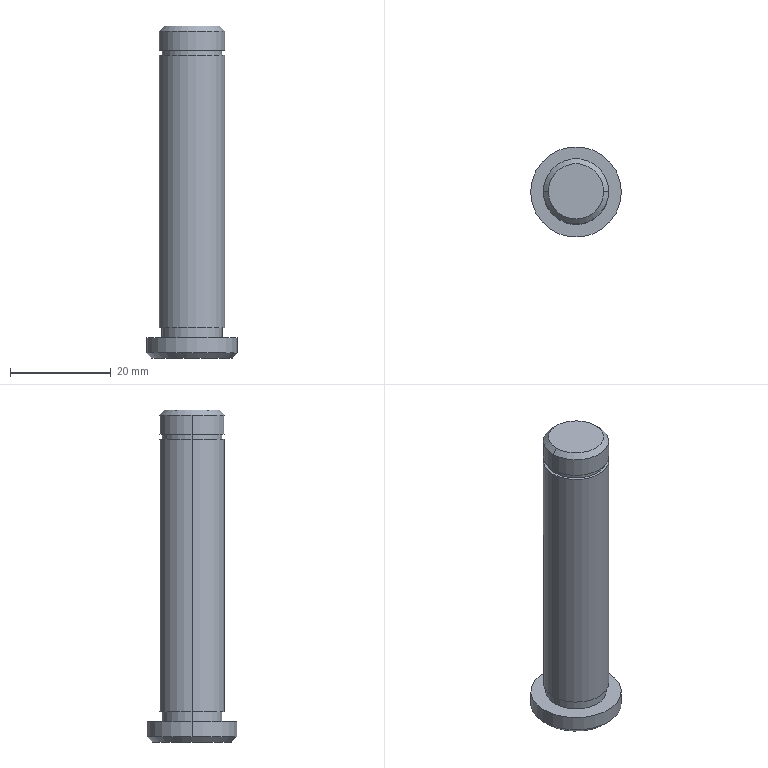Part | SolidWorks | features ICE 4, Chamfer 1, Extrusion 1 | 1 solid | 20 faces | box 18 x 18 x 66 mm | volume 9140 mm3 | cylinder 10 | plane 6 | cone 4 | commonest cylinder face diameters 13 x4 11.9 x2 12 x2 18 x2
STEP:
#1=CARTESIAN_POINT('',(5.5,0.,66.));
#2=VERTEX_POINT('',#1);
#3=CARTESIAN_POINT('',(-5.5,0.,66.));
#4=VERTEX_POINT('',#3);
#5=CARTESIAN_POINT('',(0.,0.,66.));
#6=DIRECTION('',(0.,0.,1.));
#7=DIRECTION('',(1.,0.,0.));
#8=AXIS2_PLACEMENT_3D('',#5,#6,#7);
#9=CIRCLE('',#8,5.5);
#10=EDGE_CURVE('',#2,#4,#9,.T.);
#11=ORIENTED_EDGE('',*,*,#10,.F.);
#12=CARTESIAN_POINT('',(6.5,0.,65.));
#13=VERTEX_POINT('',#12);
#14=CARTESIAN_POINT('',(5.5,0.,66.));
#15=DIRECTION('',(0.7071,0.,-0.7071));
#16=VECTOR('',#15,1000.);
#17=LINE('',#14,#16);
#18=EDGE_CURVE('',#2,#13,#17,.T.);
#19=ORIENTED_EDGE('',*,*,#18,.T.);
#20=CARTESIAN_POINT('',(-6.5,0.,65.));
#21=VERTEX_POINT('',#20);
#22=CARTESIAN_POINT('',(0.,0.,65.));
#23=DIRECTION('',(0.,0.,-1.));
#24=DIRECTION('',(1.,0.,0.));
#25=AXIS2_PLACEMENT_3D('',#22,#23,#24);
#26=CIRCLE('',#25,6.5);
#27=EDGE_CURVE('',#21,#13,#26,.T.);
#28=ORIENTED_EDGE('',*,*,#27,.F.);
#29=CARTESIAN_POINT('',(-5.5,0.,66.));
#30=DIRECTION('',(-0.7071,0.,-0.7071));
#31=VECTOR('',#30,1000.);
#32=LINE('',#29,#31);
#33=EDGE_CURVE('',#4,#21,#32,.T.);
#34=ORIENTED_EDGE('',*,*,#33,.F.);
#35=EDGE_LOOP('',(#11,#19,#28,#34));
#36=FACE_OUTER_BOUND('',#35,.T.);
#37=CARTESIAN_POINT('',(0.,0.,66.));
#38=DIRECTION('',(0.,0.,-1.));
#39=DIRECTION('',(-1.,0.,0.));
#40=AXIS2_PLACEMENT_3D('',#37,#38,#39);
#41=CONICAL_SURFACE('',#40,5.5,0.7854);
#42=ADVANCED_FACE('',(#36),#41,.T.);
#43=CARTESIAN_POINT('',(-8.,0.,0.));
#44=VERTEX_POINT('',#43);
#45=CARTESIAN_POINT('',(8.,0.,0.));
#46=VERTEX_POINT('',#45);
#47=CARTESIAN_POINT('',(0.,0.,0.));
#48=DIRECTION('',(0.,0.,-1.));
#49=DIRECTION('',(1.,0.,0.));
#50=AXIS2_PLACEMENT_3D('',#47,#48,#49);
#51=CIRCLE('',#50,8.);
#52=EDGE_CURVE('',#44,#46,#51,.T.);
#53=ORIENTED_EDGE('',*,*,#52,.F.);
#54=CARTESIAN_POINT('',(-9.,0.,1.));
#55=VERTEX_POINT('',#54);
#56=CARTESIAN_POINT('',(-9.,0.,1.));
#57=DIRECTION('',(-0.7071,0.,0.7071));
#58=VECTOR('',#57,1000.);
#59=LINE('',#56,#58);
#60=EDGE_CURVE('',#44,#55,#59,.T.);
#61=ORIENTED_EDGE('',*,*,#60,.T.);
#62=CARTESIAN_POINT('',(9.,0.,1.));
#63=VERTEX_POINT('',#62);
#64=CARTESIAN_POINT('',(0.,0.,1.));
#65=DIRECTION('',(0.,0.,1.));
#66=DIRECTION('',(1.,0.,0.));
#67=AXIS2_PLACEMENT_3D('',#64,#65,#66);
#68=CIRCLE('',#67,9.);
#69=EDGE_CURVE('',#63,#55,#68,.T.);
#70=ORIENTED_EDGE('',*,*,#69,.F.);
#71=CARTESIAN_POINT('',(9.,0.,1.));
#72=DIRECTION('',(0.7071,0.,0.7071));
#73=VECTOR('',#72,1000.);
#74=LINE('',#71,#73);
#75=EDGE_CURVE('',#46,#63,#74,.T.);
#76=ORIENTED_EDGE('',*,*,#75,.F.);
#77=EDGE_LOOP('',(#53,#61,#70,#76));
#78=FACE_OUTER_BOUND('',#77,.T.);
#79=CARTESIAN_POINT('',(0.,0.,1.));
#80=DIRECTION('',(0.,0.,1.));
#81=DIRECTION('',(1.,0.,0.));
#82=AXIS2_PLACEMENT_3D('',#79,#80,#81);
#83=CONICAL_SURFACE('',#82,9.,0.7854);
#84=ADVANCED_FACE('',(#78),#83,.T.);
#85=ORIENTED_EDGE('',*,*,#27,.T.);
#86=CARTESIAN_POINT('',(6.5,0.,61.2));
#87=VERTEX_POINT('',#86);
#88=CARTESIAN_POINT('',(6.5,0.,150.385));
#89=DIRECTION('',(0.,0.,-1.));
#90=VECTOR('',#89,1000.);
#91=LINE('',#88,#90);
#92=EDGE_CURVE('',#13,#87,#91,.T.);
#93=ORIENTED_EDGE('',*,*,#92,.T.);
#94=CARTESIAN_POINT('',(-6.5,0.,61.2));
#95=VERTEX_POINT('',#94);
#96=CARTESIAN_POINT('',(0.,0.,61.2));
#97=DIRECTION('',(0.,0.,1.));
#98=DIRECTION('',(1.,0.,0.));
#99=AXIS2_PLACEMENT_3D('',#96,#97,#98);
#100=CIRCLE('',#99,6.5);
#101=EDGE_CURVE('',#87,#95,#100,.T.);
#102=ORIENTED_EDGE('',*,*,#101,.T.);
#103=CARTESIAN_POINT('',(-6.5,0.,150.385));
#104=DIRECTION('',(0.,0.,-1.));
#105=VECTOR('',#104,1000.);
#106=LINE('',#103,#105);
#107=EDGE_CURVE('',#21,#95,#106,.T.);
#108=ORIENTED_EDGE('',*,*,#107,.F.);
#109=EDGE_LOOP('',(#85,#93,#102,#108));
#110=FACE_OUTER_BOUND('',#109,.T.);
#111=CARTESIAN_POINT('',(0.,0.,150.385));
#112=DIRECTION('',(0.,0.,-1.));
#113=DIRECTION('',(-1.,0.,0.));
#114=AXIS2_PLACEMENT_3D('',#111,#112,#113);
#115=CYLINDRICAL_SURFACE('',#114,6.5);
#116=ADVANCED_FACE('',(#110),#115,.T.);
#117=CARTESIAN_POINT('',(5.95,0.,61.2));
#118=VERTEX_POINT('',#117);
#119=CARTESIAN_POINT('',(-5.95,0.,61.2));
#120=VERTEX_POINT('',#119);
#121=CARTESIAN_POINT('',(0.,0.,61.2));
#122=DIRECTION('',(0.,0.,1.));
#123=DIRECTION('',(1.,0.,0.));
#124=AXIS2_PLACEMENT_3D('',#121,#122,#123);
#125=CIRCLE('',#124,5.95);
#126=EDGE_CURVE('',#118,#120,#125,.T.);
#127=ORIENTED_EDGE('',*,*,#126,.F.);
#128=CARTESIAN_POINT('',(5.95,0.,60.2));
#129=VERTEX_POINT('',#128);
#130=CARTESIAN_POINT('',(5.95,0.,61.2));
#131=DIRECTION('',(0.,0.,-1.));
#132=VECTOR('',#131,1000.);
#133=LINE('',#130,#132);
#134=EDGE_CURVE('',#118,#129,#133,.T.);
#135=ORIENTED_EDGE('',*,*,#134,.T.);
#136=CARTESIAN_POINT('',(-5.95,0.,60.2));
#137=VERTEX_POINT('',#136);
#138=CARTESIAN_POINT('',(0.,0.,60.2));
#139=DIRECTION('',(0.,0.,1.));
#140=DIRECTION('',(1.,0.,0.));
#141=AXIS2_PLACEMENT_3D('',#138,#139,#140);
#142=CIRCLE('',#141,5.95);
#143=EDGE_CURVE('',#129,#137,#142,.T.);
#144=ORIENTED_EDGE('',*,*,#143,.T.);
#145=CARTESIAN_POINT('',(-5.95,0.,61.2));
#146=DIRECTION('',(0.,0.,-1.));
#147=VECTOR('',#146,1000.);
#148=LINE('',#145,#147);
#149=EDGE_CURVE('',#120,#137,#148,.T.);
#150=ORIENTED_EDGE('',*,*,#149,.F.);
#151=EDGE_LOOP('',(#127,#135,#144,#150));
#152=FACE_OUTER_BOUND('',#151,.T.);
#153=CARTESIAN_POINT('',(0.,0.,61.2));
#154=DIRECTION('',(0.,0.,-1.));
#155=DIRECTION('',(-1.,0.,0.));
#156=AXIS2_PLACEMENT_3D('',#153,#154,#155);
#157=CYLINDRICAL_SURFACE('',#156,5.95);
#158=ADVANCED_FACE('',(#152),#157,.T.);
#159=CARTESIAN_POINT('',(6.5,0.,60.2));
#160=VERTEX_POINT('',#159);
#161=CARTESIAN_POINT('',(-6.5,0.,60.2));
#162=VERTEX_POINT('',#161);
#163=CARTESIAN_POINT('',(0.,0.,60.2));
#164=DIRECTION('',(0.,0.,1.));
#165=DIRECTION('',(1.,0.,0.));
#166=AXIS2_PLACEMENT_3D('',#163,#164,#165);
#167=CIRCLE('',#166,6.5);
#168=EDGE_CURVE('',#160,#162,#167,.T.);
#169=ORIENTED_EDGE('',*,*,#168,.F.);
#170=CARTESIAN_POINT('',(6.5,0.,6.));
#171=VERTEX_POINT('',#170);
#172=CARTESIAN_POINT('',(6.5,0.,60.2));
#173=DIRECTION('',(0.,0.,-1.));
#174=VECTOR('',#173,1000.);
#175=LINE('',#172,#174);
#176=EDGE_CURVE('',#160,#171,#175,.T.);
#177=ORIENTED_EDGE('',*,*,#176,.T.);
#178=CARTESIAN_POINT('',(-6.5,0.,6.));
#179=VERTEX_POINT('',#178);
#180=CARTESIAN_POINT('',(0.,0.,6.));
#181=DIRECTION('',(0.,0.,1.));
#182=DIRECTION('',(1.,0.,0.));
#183=AXIS2_PLACEMENT_3D('',#180,#181,#182);
#184=CIRCLE('',#183,6.5);
#185=EDGE_CURVE('',#171,#179,#184,.T.);
#186=ORIENTED_EDGE('',*,*,#185,.T.);
#187=CARTESIAN_POINT('',(-6.5,0.,60.2));
#188=DIRECTION('',(0.,0.,-1.));
#189=VECTOR('',#188,1000.);
#190=LINE('',#187,#189);
#191=EDGE_CURVE('',#162,#179,#190,.T.);
#192=ORIENTED_EDGE('',*,*,#191,.F.);
#193=EDGE_LOOP('',(#169,#177,#186,#192));
#194=FACE_OUTER_BOUND('',#193,.T.);
#195=CARTESIAN_POINT('',(0.,0.,60.2));
#196=DIRECTION('',(0.,0.,-1.));
#197=DIRECTION('',(-1.,0.,0.));
#198=AXIS2_PLACEMENT_3D('',#195,#196,#197);
#199=CYLINDRICAL_SURFACE('',#198,6.5);
#200=ADVANCED_FACE('',(#194),#199,.T.);
#201=CARTESIAN_POINT('',(6.,0.,6.));
#202=VERTEX_POINT('',#201);
#203=CARTESIAN_POINT('',(-6.,0.,6.));
#204=VERTEX_POINT('',#203);
#205=CARTESIAN_POINT('',(0.,0.,6.));
#206=DIRECTION('',(0.,0.,1.));
#207=DIRECTION('',(1.,0.,0.));
#208=AXIS2_PLACEMENT_3D('',#205,#206,#207);
#209=CIRCLE('',#208,6.);
#210=EDGE_CURVE('',#202,#204,#209,.T.);
#211=ORIENTED_EDGE('',*,*,#210,.F.);
#212=CARTESIAN_POINT('',(6.,0.,4.));
#213=VERTEX_POINT('',#212);
#214=CARTESIAN_POINT('',(6.,0.,6.));
#215=DIRECTION('',(0.,0.,-1.));
#216=VECTOR('',#215,1000.);
#217=LINE('',#214,#216);
#218=EDGE_CURVE('',#202,#213,#217,.T.);
#219=ORIENTED_EDGE('',*,*,#218,.T.);
#220=CARTESIAN_POINT('',(-6.,0.,4.));
#221=VERTEX_POINT('',#220);
#222=CARTESIAN_POINT('',(0.,0.,4.));
#223=DIRECTION('',(0.,0.,1.));
#224=DIRECTION('',(1.,0.,0.));
#225=AXIS2_PLACEMENT_3D('',#222,#223,#224);
#226=CIRCLE('',#225,6.);
#227=EDGE_CURVE('',#213,#221,#226,.T.);
#228=ORIENTED_EDGE('',*,*,#227,.T.);
#229=CARTESIAN_POINT('',(-6.,0.,6.));
#230=DIRECTION('',(0.,0.,-1.));
#231=VECTOR('',#230,1000.);
#232=LINE('',#229,#231);
#233=EDGE_CURVE('',#204,#221,#232,.T.);
#234=ORIENTED_EDGE('',*,*,#233,.F.);
#235=EDGE_LOOP('',(#211,#219,#228,#234));
#236=FACE_OUTER_BOUND('',#235,.T.);
#237=CARTESIAN_POINT('',(0.,0.,6.));
#238=DIRECTION('',(0.,0.,-1.));
#239=DIRECTION('',(-1.,0.,0.));
#240=AXIS2_PLACEMENT_3D('',#237,#238,#239);
#241=CYLINDRICAL_SURFACE('',#240,6.);
#242=ADVANCED_FACE('',(#236),#241,.T.);
#243=CARTESIAN_POINT('',(9.,0.,4.));
#244=VERTEX_POINT('',#243);
#245=CARTESIAN_POINT('',(-9.,0.,4.));
#246=VERTEX_POINT('',#245);
#247=CARTESIAN_POINT('',(0.,0.,4.));
#248=DIRECTION('',(0.,0.,1.));
#249=DIRECTION('',(1.,0.,0.));
#250=AXIS2_PLACEMENT_3D('',#247,#248,#249);
#251=CIRCLE('',#250,9.);
#252=EDGE_CURVE('',#244,#246,#251,.T.);
#253=ORIENTED_EDGE('',*,*,#252,.F.);
#254=CARTESIAN_POINT('',(9.,0.,4.));
#255=DIRECTION('',(0.,0.,-1.));
#256=VECTOR('',#255,1000.);
#257=LINE('',#254,#256);
#258=EDGE_CURVE('',#244,#63,#257,.T.);
#259=ORIENTED_EDGE('',*,*,#258,.T.);
#260=ORIENTED_EDGE('',*,*,#69,.T.);
#261=CARTESIAN_POINT('',(-9.,0.,4.));
#262=DIRECTION('',(0.,0.,-1.));
#263=VECTOR('',#262,1000.);
#264=LINE('',#261,#263);
#265=EDGE_CURVE('',#246,#55,#264,.T.);
#266=ORIENTED_EDGE('',*,*,#265,.F.);
#267=EDGE_LOOP('',(#253,#259,#260,#266));
#268=FACE_OUTER_BOUND('',#267,.T.);
#269=CARTESIAN_POINT('',(0.,0.,4.));
#270=DIRECTION('',(0.,0.,-1.));
#271=DIRECTION('',(-1.,0.,0.));
#272=AXIS2_PLACEMENT_3D('',#269,#270,#271);
#273=CYLINDRICAL_SURFACE('',#272,9.);
#274=ADVANCED_FACE('',(#268),#273,.T.);
#275=ORIENTED_EDGE('',*,*,#258,.F.);
#276=CARTESIAN_POINT('',(0.,0.,4.));
#277=DIRECTION('',(0.,0.,1.));
#278=DIRECTION('',(1.,0.,0.));
#279=AXIS2_PLACEMENT_3D('',#276,#277,#278);
#280=CIRCLE('',#279,9.);
#281=EDGE_CURVE('',#246,#244,#280,.T.);
#282=ORIENTED_EDGE('',*,*,#281,.F.);
#283=ORIENTED_EDGE('',*,*,#265,.T.);
#284=CARTESIAN_POINT('',(0.,0.,1.));
#285=DIRECTION('',(0.,0.,1.));
#286=DIRECTION('',(1.,0.,0.));
#287=AXIS2_PLACEMENT_3D('',#284,#285,#286);
#288=CIRCLE('',#287,9.);
#289=EDGE_CURVE('',#55,#63,#288,.T.);
#290=ORIENTED_EDGE('',*,*,#289,.T.);
#291=EDGE_LOOP('',(#275,#282,#283,#290));
#292=FACE_OUTER_BOUND('',#291,.T.);
#293=CARTESIAN_POINT('',(0.,0.,4.));
#294=DIRECTION('',(0.,0.,-1.));
#295=DIRECTION('',(-1.,0.,0.));
#296=AXIS2_PLACEMENT_3D('',#293,#294,#295);
#297=CYLINDRICAL_SURFACE('',#296,9.);
#298=ADVANCED_FACE('',(#292),#297,.T.);
#299=CARTESIAN_POINT('',(0.,0.,4.));
#300=DIRECTION('',(0.,0.,1.));
#301=DIRECTION('',(1.,0.,0.));
#302=AXIS2_PLACEMENT_3D('',#299,#300,#301);
#303=CIRCLE('',#302,6.);
#304=EDGE_CURVE('',#221,#213,#303,.T.);
#305=ORIENTED_EDGE('',*,*,#304,.F.);
#306=ORIENTED_EDGE('',*,*,#227,.F.);
#307=EDGE_LOOP('',(#305,#306));
#308=FACE_BOUND('',#307,.T.);
#309=ORIENTED_EDGE('',*,*,#281,.T.);
#310=ORIENTED_EDGE('',*,*,#252,.T.);
#311=EDGE_LOOP('',(#309,#310));
#312=FACE_OUTER_BOUND('',#311,.T.);
#313=CARTESIAN_POINT('',(0.,0.,4.));
#314=DIRECTION('',(0.,0.,1.));
#315=DIRECTION('',(1.,0.,0.));
#316=AXIS2_PLACEMENT_3D('',#313,#314,#315);
#317=PLANE('',#316);
#318=ADVANCED_FACE('',(#308,#312),#317,.T.);
#319=CARTESIAN_POINT('',(0.,0.,0.));
#320=DIRECTION('',(0.,0.,-1.));
#321=DIRECTION('',(1.,0.,0.));
#322=AXIS2_PLACEMENT_3D('',#319,#320,#321);
#323=CIRCLE('',#322,8.);
#324=EDGE_CURVE('',#46,#44,#323,.T.);
#325=ORIENTED_EDGE('',*,*,#324,.T.);
#326=ORIENTED_EDGE('',*,*,#52,.T.);
#327=EDGE_LOOP('',(#325,#326));
#328=FACE_OUTER_BOUND('',#327,.T.);
#329=CARTESIAN_POINT('',(0.,0.,0.));
#330=DIRECTION('',(0.,0.,1.));
#331=DIRECTION('',(1.,0.,0.));
#332=AXIS2_PLACEMENT_3D('',#329,#330,#331);
#333=PLANE('',#332);
#334=ADVANCED_FACE('',(#328),#333,.F.);
#335=ORIENTED_EDGE('',*,*,#218,.F.);
#336=CARTESIAN_POINT('',(0.,0.,6.));
#337=DIRECTION('',(0.,0.,1.));
#338=DIRECTION('',(1.,0.,0.));
#339=AXIS2_PLACEMENT_3D('',#336,#337,#338);
#340=CIRCLE('',#339,6.);
#341=EDGE_CURVE('',#204,#202,#340,.T.);
#342=ORIENTED_EDGE('',*,*,#341,.F.);
#343=ORIENTED_EDGE('',*,*,#233,.T.);
#344=ORIENTED_EDGE('',*,*,#304,.T.);
#345=EDGE_LOOP('',(#335,#342,#343,#344));
#346=FACE_OUTER_BOUND('',#345,.T.);
#347=CARTESIAN_POINT('',(0.,0.,6.));
#348=DIRECTION('',(0.,0.,-1.));
#349=DIRECTION('',(-1.,0.,0.));
#350=AXIS2_PLACEMENT_3D('',#347,#348,#349);
#351=CYLINDRICAL_SURFACE('',#350,6.);
#352=ADVANCED_FACE('',(#346),#351,.T.);
#353=ORIENTED_EDGE('',*,*,#176,.F.);
#354=CARTESIAN_POINT('',(0.,0.,60.2));
#355=DIRECTION('',(0.,0.,1.));
#356=DIRECTION('',(1.,0.,0.));
#357=AXIS2_PLACEMENT_3D('',#354,#355,#356);
#358=CIRCLE('',#357,6.5);
#359=EDGE_CURVE('',#162,#160,#358,.T.);
#360=ORIENTED_EDGE('',*,*,#359,.F.);
#361=ORIENTED_EDGE('',*,*,#191,.T.);
#362=CARTESIAN_POINT('',(0.,0.,6.));
#363=DIRECTION('',(0.,0.,1.));
#364=DIRECTION('',(1.,0.,0.));
#365=AXIS2_PLACEMENT_3D('',#362,#363,#364);
#366=CIRCLE('',#365,6.5);
#367=EDGE_CURVE('',#179,#171,#366,.T.);
#368=ORIENTED_EDGE('',*,*,#367,.T.);
#369=EDGE_LOOP('',(#353,#360,#361,#368));
#370=FACE_OUTER_BOUND('',#369,.T.);
#371=CARTESIAN_POINT('',(0.,0.,60.2));
#372=DIRECTION('',(0.,0.,-1.));
#373=DIRECTION('',(-1.,0.,0.));
#374=AXIS2_PLACEMENT_3D('',#371,#372,#373);
#375=CYLINDRICAL_SURFACE('',#374,6.5);
#376=ADVANCED_FACE('',(#370),#375,.T.);
#377=CARTESIAN_POINT('',(0.,0.,60.2));
#378=DIRECTION('',(0.,0.,1.));
#379=DIRECTION('',(1.,0.,0.));
#380=AXIS2_PLACEMENT_3D('',#377,#378,#379);
#381=CIRCLE('',#380,5.95);
#382=EDGE_CURVE('',#137,#129,#381,.T.);
#383=ORIENTED_EDGE('',*,*,#382,.F.);
#384=ORIENTED_EDGE('',*,*,#143,.F.);
#385=EDGE_LOOP('',(#383,#384));
#386=FACE_BOUND('',#385,.T.);
#387=ORIENTED_EDGE('',*,*,#359,.T.);
#388=ORIENTED_EDGE('',*,*,#168,.T.);
#389=EDGE_LOOP('',(#387,#388));
#390=FACE_OUTER_BOUND('',#389,.T.);
#391=CARTESIAN_POINT('',(0.,0.,60.2));
#392=DIRECTION('',(0.,0.,1.));
#393=DIRECTION('',(1.,0.,0.));
#394=AXIS2_PLACEMENT_3D('',#391,#392,#393);
#395=PLANE('',#394);
#396=ADVANCED_FACE('',(#386,#390),#395,.T.);
#397=ORIENTED_EDGE('',*,*,#341,.T.);
#398=ORIENTED_EDGE('',*,*,#210,.T.);
#399=EDGE_LOOP('',(#397,#398));
#400=FACE_BOUND('',#399,.T.);
#401=ORIENTED_EDGE('',*,*,#367,.F.);
#402=ORIENTED_EDGE('',*,*,#185,.F.);
#403=EDGE_LOOP('',(#401,#402));
#404=FACE_OUTER_BOUND('',#403,.T.);
#405=CARTESIAN_POINT('',(0.,0.,6.));
#406=DIRECTION('',(0.,0.,1.));
#407=DIRECTION('',(1.,0.,0.));
#408=AXIS2_PLACEMENT_3D('',#405,#406,#407);
#409=PLANE('',#408);
#410=ADVANCED_FACE('',(#400,#404),#409,.F.);
#411=ORIENTED_EDGE('',*,*,#134,.F.);
#412=CARTESIAN_POINT('',(0.,0.,61.2));
#413=DIRECTION('',(0.,0.,1.));
#414=DIRECTION('',(1.,0.,0.));
#415=AXIS2_PLACEMENT_3D('',#412,#413,#414);
#416=CIRCLE('',#415,5.95);
#417=EDGE_CURVE('',#120,#118,#416,.T.);
#418=ORIENTED_EDGE('',*,*,#417,.F.);
#419=ORIENTED_EDGE('',*,*,#149,.T.);
#420=ORIENTED_EDGE('',*,*,#382,.T.);
#421=EDGE_LOOP('',(#411,#418,#419,#420));
#422=FACE_OUTER_BOUND('',#421,.T.);
#423=CARTESIAN_POINT('',(0.,0.,61.2));
#424=DIRECTION('',(0.,0.,-1.));
#425=DIRECTION('',(-1.,0.,0.));
#426=AXIS2_PLACEMENT_3D('',#423,#424,#425);
#427=CYLINDRICAL_SURFACE('',#426,5.95);
#428=ADVANCED_FACE('',(#422),#427,.T.);
#429=ORIENTED_EDGE('',*,*,#92,.F.);
#430=CARTESIAN_POINT('',(0.,0.,65.));
#431=DIRECTION('',(0.,0.,-1.));
#432=DIRECTION('',(1.,0.,0.));
#433=AXIS2_PLACEMENT_3D('',#430,#431,#432);
#434=CIRCLE('',#433,6.5);
#435=EDGE_CURVE('',#13,#21,#434,.T.);
#436=ORIENTED_EDGE('',*,*,#435,.T.);
#437=ORIENTED_EDGE('',*,*,#107,.T.);
#438=CARTESIAN_POINT('',(0.,0.,61.2));
#439=DIRECTION('',(0.,0.,1.));
#440=DIRECTION('',(1.,0.,0.));
#441=AXIS2_PLACEMENT_3D('',#438,#439,#440);
#442=CIRCLE('',#441,6.5);
#443=EDGE_CURVE('',#95,#87,#442,.T.);
#444=ORIENTED_EDGE('',*,*,#443,.T.);
#445=EDGE_LOOP('',(#429,#436,#437,#444));
#446=FACE_OUTER_BOUND('',#445,.T.);
#447=CARTESIAN_POINT('',(0.,0.,150.385));
#448=DIRECTION('',(0.,0.,-1.));
#449=DIRECTION('',(-1.,0.,0.));
#450=AXIS2_PLACEMENT_3D('',#447,#448,#449);
#451=CYLINDRICAL_SURFACE('',#450,6.5);
#452=ADVANCED_FACE('',(#446),#451,.T.);
#453=ORIENTED_EDGE('',*,*,#417,.T.);
#454=ORIENTED_EDGE('',*,*,#126,.T.);
#455=EDGE_LOOP('',(#453,#454));
#456=FACE_BOUND('',#455,.T.);
#457=ORIENTED_EDGE('',*,*,#443,.F.);
#458=ORIENTED_EDGE('',*,*,#101,.F.);
#459=EDGE_LOOP('',(#457,#458));
#460=FACE_OUTER_BOUND('',#459,.T.);
#461=CARTESIAN_POINT('',(0.,0.,61.2));
#462=DIRECTION('',(0.,0.,1.));
#463=DIRECTION('',(1.,0.,0.));
#464=AXIS2_PLACEMENT_3D('',#461,#462,#463);
#465=PLANE('',#464);
#466=ADVANCED_FACE('',(#456,#460),#465,.F.);
#467=CARTESIAN_POINT('',(0.,0.,66.));
#468=DIRECTION('',(0.,0.,1.));
#469=DIRECTION('',(1.,0.,0.));
#470=AXIS2_PLACEMENT_3D('',#467,#468,#469);
#471=CIRCLE('',#470,5.5);
#472=EDGE_CURVE('',#4,#2,#471,.T.);
#473=ORIENTED_EDGE('',*,*,#472,.T.);
#474=ORIENTED_EDGE('',*,*,#10,.T.);
#475=EDGE_LOOP('',(#473,#474));
#476=FACE_OUTER_BOUND('',#475,.T.);
#477=CARTESIAN_POINT('',(0.,0.,66.));
#478=DIRECTION('',(0.,0.,1.));
#479=DIRECTION('',(1.,0.,0.));
#480=AXIS2_PLACEMENT_3D('',#477,#478,#479);
#481=PLANE('',#480);
#482=ADVANCED_FACE('',(#476),#481,.T.);
#483=ORIENTED_EDGE('',*,*,#60,.F.);
#484=ORIENTED_EDGE('',*,*,#324,.F.);
#485=ORIENTED_EDGE('',*,*,#75,.T.);
#486=ORIENTED_EDGE('',*,*,#289,.F.);
#487=EDGE_LOOP('',(#483,#484,#485,#486));
#488=FACE_OUTER_BOUND('',#487,.T.);
#489=CARTESIAN_POINT('',(0.,0.,1.));
#490=DIRECTION('',(0.,0.,1.));
#491=DIRECTION('',(1.,0.,0.));
#492=AXIS2_PLACEMENT_3D('',#489,#490,#491);
#493=CONICAL_SURFACE('',#492,9.,0.7854);
#494=ADVANCED_FACE('',(#488),#493,.T.);
#495=ORIENTED_EDGE('',*,*,#18,.F.);
#496=ORIENTED_EDGE('',*,*,#472,.F.);
#497=ORIENTED_EDGE('',*,*,#33,.T.);
#498=ORIENTED_EDGE('',*,*,#435,.F.);
#499=EDGE_LOOP('',(#495,#496,#497,#498));
#500=FACE_OUTER_BOUND('',#499,.T.);
#501=CARTESIAN_POINT('',(0.,0.,66.));
#502=DIRECTION('',(0.,0.,-1.));
#503=DIRECTION('',(-1.,0.,0.));
#504=AXIS2_PLACEMENT_3D('',#501,#502,#503);
#505=CONICAL_SURFACE('',#504,5.5,0.7854);
#506=ADVANCED_FACE('',(#500),#505,.T.);
#507=CLOSED_SHELL('',(#42,#84,#116,#158,#200,#242,#274,#298,#318,#334,#352,#376,#396,#410,#428,#452,#466,#482,#494,#506));
#508=MANIFOLD_SOLID_BREP('',#507);
#509=CARTESIAN_POINT('',(0.,0.,0.));
#510=DIRECTION('',(0.,0.,1.));
#511=DIRECTION('',(1.,0.,0.));
#512=AXIS2_PLACEMENT_3D('',#509,#510,#511);
#513=(LENGTH_UNIT()NAMED_UNIT(*)SI_UNIT(.MILLI.,.METRE.));
#514=UNCERTAINTY_MEASURE_WITH_UNIT(LENGTH_MEASURE(0.00001),#513,'','');
#515=(NAMED_UNIT(*)PLANE_ANGLE_UNIT()SI_UNIT($,.RADIAN.));
#516=(NAMED_UNIT(*)SI_UNIT($,.STERADIAN.)SOLID_ANGLE_UNIT());
#517=(GEOMETRIC_REPRESENTATION_CONTEXT(3)GLOBAL_UNCERTAINTY_ASSIGNED_CONTEXT((#514))GLOBAL_UNIT_ASSIGNED_CONTEXT((#513,#515,#516))REPRESENTATION_CONTEXT('',''));
#518=ADVANCED_BREP_SHAPE_REPRESENTATION('',(#508,#512),#517);